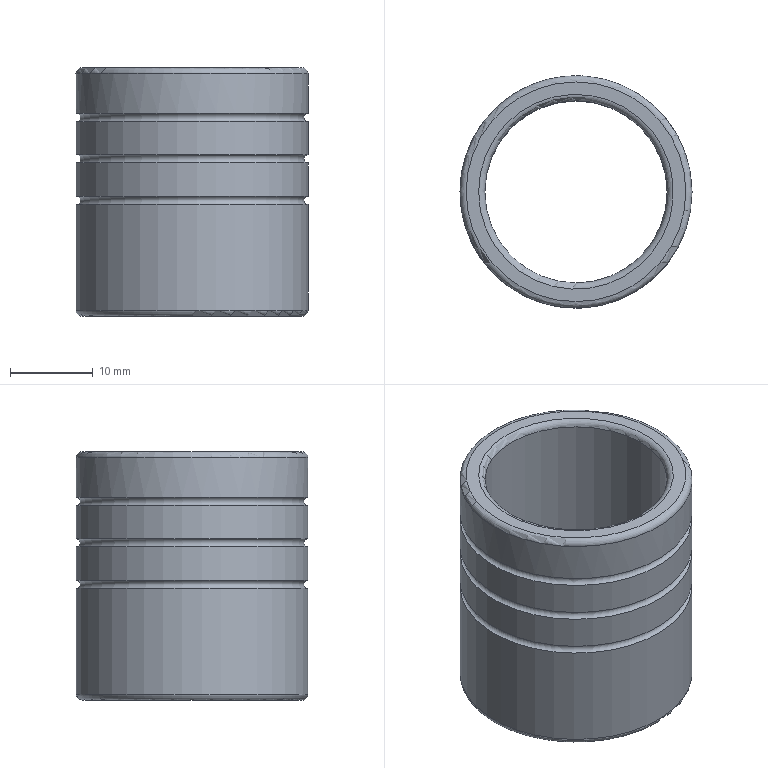Part | STEP file | 200 mesh_id1790 | 1 solid | 14 faces | box 28 x 28 x 30 mm | volume 6929 mm3 | torus 7 | cylinder 5 | plane 2 | commonest cylinder face diameters 28 x4 22 x1
STEP:
#1=CARTESIAN_POINT('',(-17063.884,-4095.269,123.508));
#2=VERTEX_POINT('',#1);
#3=CARTESIAN_POINT('',(-17052.884,-4095.269,123.508));
#4=DIRECTION('',(0.,0.,1.));
#5=DIRECTION('',(-1.,0.,0.));
#6=AXIS2_PLACEMENT_3D('',#3,#4,#5);
#7=CIRCLE('',#6,11.);
#8=EDGE_CURVE('',#2,#2,#7,.T.);
#9=ORIENTED_EDGE('',*,*,#8,.T.);
#10=EDGE_LOOP('',(#9));
#11=FACE_BOUND('',#10,.T.);
#12=CARTESIAN_POINT('',(-17041.884,-4095.269,95.008));
#13=VERTEX_POINT('',#12);
#14=CARTESIAN_POINT('',(-17052.884,-4095.269,95.008));
#15=DIRECTION('',(0.,0.,-1.));
#16=DIRECTION('',(1.,0.,0.));
#17=AXIS2_PLACEMENT_3D('',#14,#15,#16);
#18=CIRCLE('',#17,11.);
#19=EDGE_CURVE('',#13,#13,#18,.T.);
#20=ORIENTED_EDGE('',*,*,#19,.T.);
#21=EDGE_LOOP('',(#20));
#22=FACE_BOUND('',#21,.T.);
#23=CARTESIAN_POINT('',(-17052.884,-4095.269,79.258));
#24=DIRECTION('',(0.,0.,1.));
#25=DIRECTION('',(1.,0.,0.));
#26=AXIS2_PLACEMENT_3D('',#23,#24,#25);
#27=CYLINDRICAL_SURFACE('',#26,11.);
#28=ADVANCED_FACE('',(#11,#22),#27,.F.);
#29=CARTESIAN_POINT('',(-17039.634,-4095.269,94.258));
#30=VERTEX_POINT('',#29);
#31=CARTESIAN_POINT('',(-17052.884,-4095.269,94.258));
#32=DIRECTION('',(0.,0.,-1.));
#33=DIRECTION('',(1.,0.,0.));
#34=AXIS2_PLACEMENT_3D('',#31,#32,#33);
#35=CIRCLE('',#34,13.25);
#36=EDGE_CURVE('',#30,#30,#35,.T.);
#37=ORIENTED_EDGE('',*,*,#36,.T.);
#38=EDGE_LOOP('',(#37));
#39=FACE_BOUND('',#38,.T.);
#40=CARTESIAN_POINT('',(-17041.134,-4095.269,94.258));
#41=VERTEX_POINT('',#40);
#42=CARTESIAN_POINT('',(-17052.884,-4095.269,94.258));
#43=DIRECTION('',(0.,0.,1.));
#44=DIRECTION('',(1.,0.,0.));
#45=AXIS2_PLACEMENT_3D('',#42,#43,#44);
#46=CIRCLE('',#45,11.75);
#47=EDGE_CURVE('',#41,#41,#46,.T.);
#48=ORIENTED_EDGE('',*,*,#47,.T.);
#49=EDGE_LOOP('',(#48));
#50=FACE_BOUND('',#49,.T.);
#51=CARTESIAN_POINT('',(-17063.884,-4095.269,94.258));
#52=DIRECTION('',(0.,0.,1.));
#53=DIRECTION('',(1.,0.,0.));
#54=AXIS2_PLACEMENT_3D('',#51,#52,#53);
#55=PLANE('',#54);
#56=ADVANCED_FACE('',(#39,#50),#55,.F.);
#57=CARTESIAN_POINT('',(-17038.884,-4095.269,95.008));
#58=VERTEX_POINT('',#57);
#59=CARTESIAN_POINT('',(-17052.884,-4095.269,95.008));
#60=DIRECTION('',(0.,0.,1.));
#61=DIRECTION('',(1.,0.,0.));
#62=AXIS2_PLACEMENT_3D('',#59,#60,#61);
#63=CIRCLE('',#62,14.);
#64=EDGE_CURVE('',#58,#58,#63,.T.);
#65=ORIENTED_EDGE('',*,*,#64,.T.);
#66=EDGE_LOOP('',(#65));
#67=FACE_BOUND('',#66,.T.);
#68=CARTESIAN_POINT('',(-17038.884,-4095.269,107.758));
#69=VERTEX_POINT('',#68);
#70=CARTESIAN_POINT('',(-17052.884,-4095.269,107.758));
#71=DIRECTION('',(0.,0.,1.));
#72=DIRECTION('',(1.,0.,0.));
#73=AXIS2_PLACEMENT_3D('',#70,#71,#72);
#74=CIRCLE('',#73,14.);
#75=EDGE_CURVE('',#69,#69,#74,.T.);
#76=ORIENTED_EDGE('',*,*,#75,.F.);
#77=EDGE_LOOP('',(#76));
#78=FACE_BOUND('',#77,.T.);
#79=CARTESIAN_POINT('',(-17052.884,-4095.269,79.258));
#80=DIRECTION('',(0.,0.,1.));
#81=DIRECTION('',(1.,0.,0.));
#82=AXIS2_PLACEMENT_3D('',#79,#80,#81);
#83=CYLINDRICAL_SURFACE('',#82,14.);
#84=ADVANCED_FACE('',(#67,#78),#83,.T.);
#85=CARTESIAN_POINT('',(-17038.884,-4095.269,108.758));
#86=VERTEX_POINT('',#85);
#87=CARTESIAN_POINT('',(-17052.884,-4095.269,108.758));
#88=DIRECTION('',(0.,0.,1.));
#89=DIRECTION('',(1.,0.,0.));
#90=AXIS2_PLACEMENT_3D('',#87,#88,#89);
#91=CIRCLE('',#90,14.);
#92=EDGE_CURVE('',#86,#86,#91,.T.);
#93=ORIENTED_EDGE('',*,*,#92,.F.);
#94=EDGE_LOOP('',(#93));
#95=FACE_BOUND('',#94,.T.);
#96=ORIENTED_EDGE('',*,*,#75,.T.);
#97=EDGE_LOOP('',(#96));
#98=FACE_BOUND('',#97,.T.);
#99=CARTESIAN_POINT('',(-17052.884,-4095.269,108.258));
#100=DIRECTION('',(0.,0.,1.));
#101=DIRECTION('',(1.,0.,0.));
#102=AXIS2_PLACEMENT_3D('',#99,#100,#101);
#103=TOROIDAL_SURFACE('',#102,14.,0.5);
#104=ADVANCED_FACE('',(#95,#98),#103,.F.);
#105=CARTESIAN_POINT('',(-17038.884,-4095.269,112.758));
#106=VERTEX_POINT('',#105);
#107=CARTESIAN_POINT('',(-17052.884,-4095.269,112.758));
#108=DIRECTION('',(0.,0.,1.));
#109=DIRECTION('',(1.,0.,0.));
#110=AXIS2_PLACEMENT_3D('',#107,#108,#109);
#111=CIRCLE('',#110,14.);
#112=EDGE_CURVE('',#106,#106,#111,.T.);
#113=ORIENTED_EDGE('',*,*,#112,.F.);
#114=EDGE_LOOP('',(#113));
#115=FACE_BOUND('',#114,.T.);
#116=ORIENTED_EDGE('',*,*,#92,.T.);
#117=EDGE_LOOP('',(#116));
#118=FACE_BOUND('',#117,.T.);
#119=CARTESIAN_POINT('',(-17052.884,-4095.269,79.258));
#120=DIRECTION('',(0.,0.,1.));
#121=DIRECTION('',(1.,0.,0.));
#122=AXIS2_PLACEMENT_3D('',#119,#120,#121);
#123=CYLINDRICAL_SURFACE('',#122,14.);
#124=ADVANCED_FACE('',(#115,#118),#123,.T.);
#125=CARTESIAN_POINT('',(-17038.884,-4095.269,113.758));
#126=VERTEX_POINT('',#125);
#127=CARTESIAN_POINT('',(-17052.884,-4095.269,113.758));
#128=DIRECTION('',(0.,0.,1.));
#129=DIRECTION('',(1.,0.,0.));
#130=AXIS2_PLACEMENT_3D('',#127,#128,#129);
#131=CIRCLE('',#130,14.);
#132=EDGE_CURVE('',#126,#126,#131,.T.);
#133=ORIENTED_EDGE('',*,*,#132,.F.);
#134=EDGE_LOOP('',(#133));
#135=FACE_BOUND('',#134,.T.);
#136=ORIENTED_EDGE('',*,*,#112,.T.);
#137=EDGE_LOOP('',(#136));
#138=FACE_BOUND('',#137,.T.);
#139=CARTESIAN_POINT('',(-17052.884,-4095.269,113.258));
#140=DIRECTION('',(0.,0.,1.));
#141=DIRECTION('',(1.,0.,0.));
#142=AXIS2_PLACEMENT_3D('',#139,#140,#141);
#143=TOROIDAL_SURFACE('',#142,14.,0.5);
#144=ADVANCED_FACE('',(#135,#138),#143,.F.);
#145=CARTESIAN_POINT('',(-17038.884,-4095.269,117.758));
#146=VERTEX_POINT('',#145);
#147=CARTESIAN_POINT('',(-17052.884,-4095.269,117.758));
#148=DIRECTION('',(0.,0.,1.));
#149=DIRECTION('',(1.,0.,0.));
#150=AXIS2_PLACEMENT_3D('',#147,#148,#149);
#151=CIRCLE('',#150,14.);
#152=EDGE_CURVE('',#146,#146,#151,.T.);
#153=ORIENTED_EDGE('',*,*,#152,.F.);
#154=EDGE_LOOP('',(#153));
#155=FACE_BOUND('',#154,.T.);
#156=ORIENTED_EDGE('',*,*,#132,.T.);
#157=EDGE_LOOP('',(#156));
#158=FACE_BOUND('',#157,.T.);
#159=CARTESIAN_POINT('',(-17052.884,-4095.269,79.258));
#160=DIRECTION('',(0.,0.,1.));
#161=DIRECTION('',(1.,0.,0.));
#162=AXIS2_PLACEMENT_3D('',#159,#160,#161);
#163=CYLINDRICAL_SURFACE('',#162,14.);
#164=ADVANCED_FACE('',(#155,#158),#163,.T.);
#165=CARTESIAN_POINT('',(-17038.884,-4095.269,118.758));
#166=VERTEX_POINT('',#165);
#167=CARTESIAN_POINT('',(-17052.884,-4095.269,118.758));
#168=DIRECTION('',(0.,0.,1.));
#169=DIRECTION('',(1.,0.,0.));
#170=AXIS2_PLACEMENT_3D('',#167,#168,#169);
#171=CIRCLE('',#170,14.);
#172=EDGE_CURVE('',#166,#166,#171,.T.);
#173=ORIENTED_EDGE('',*,*,#172,.F.);
#174=EDGE_LOOP('',(#173));
#175=FACE_BOUND('',#174,.T.);
#176=ORIENTED_EDGE('',*,*,#152,.T.);
#177=EDGE_LOOP('',(#176));
#178=FACE_BOUND('',#177,.T.);
#179=CARTESIAN_POINT('',(-17052.884,-4095.269,118.258));
#180=DIRECTION('',(0.,0.,1.));
#181=DIRECTION('',(1.,0.,0.));
#182=AXIS2_PLACEMENT_3D('',#179,#180,#181);
#183=TOROIDAL_SURFACE('',#182,14.,0.5);
#184=ADVANCED_FACE('',(#175,#178),#183,.F.);
#185=CARTESIAN_POINT('',(-17066.884,-4095.269,123.508));
#186=VERTEX_POINT('',#185);
#187=CARTESIAN_POINT('',(-17052.884,-4095.269,123.508));
#188=DIRECTION('',(0.,0.,-1.));
#189=DIRECTION('',(-1.,0.,0.));
#190=AXIS2_PLACEMENT_3D('',#187,#188,#189);
#191=CIRCLE('',#190,14.);
#192=EDGE_CURVE('',#186,#186,#191,.T.);
#193=ORIENTED_EDGE('',*,*,#192,.T.);
#194=EDGE_LOOP('',(#193));
#195=FACE_BOUND('',#194,.T.);
#196=ORIENTED_EDGE('',*,*,#172,.T.);
#197=EDGE_LOOP('',(#196));
#198=FACE_BOUND('',#197,.T.);
#199=CARTESIAN_POINT('',(-17052.884,-4095.269,79.258));
#200=DIRECTION('',(0.,0.,1.));
#201=DIRECTION('',(1.,0.,0.));
#202=AXIS2_PLACEMENT_3D('',#199,#200,#201);
#203=CYLINDRICAL_SURFACE('',#202,14.);
#204=ADVANCED_FACE('',(#195,#198),#203,.T.);
#205=CARTESIAN_POINT('',(-17064.634,-4095.269,124.258));
#206=VERTEX_POINT('',#205);
#207=CARTESIAN_POINT('',(-17052.884,-4095.269,124.258));
#208=DIRECTION('',(0.,0.,-1.));
#209=DIRECTION('',(-1.,0.,0.));
#210=AXIS2_PLACEMENT_3D('',#207,#208,#209);
#211=CIRCLE('',#210,11.75);
#212=EDGE_CURVE('',#206,#206,#211,.T.);
#213=ORIENTED_EDGE('',*,*,#212,.T.);
#214=EDGE_LOOP('',(#213));
#215=FACE_BOUND('',#214,.T.);
#216=CARTESIAN_POINT('',(-17066.134,-4095.269,124.258));
#217=VERTEX_POINT('',#216);
#218=CARTESIAN_POINT('',(-17052.884,-4095.269,124.258));
#219=DIRECTION('',(0.,0.,1.));
#220=DIRECTION('',(-1.,0.,0.));
#221=AXIS2_PLACEMENT_3D('',#218,#219,#220);
#222=CIRCLE('',#221,13.25);
#223=EDGE_CURVE('',#217,#217,#222,.T.);
#224=ORIENTED_EDGE('',*,*,#223,.T.);
#225=EDGE_LOOP('',(#224));
#226=FACE_BOUND('',#225,.T.);
#227=CARTESIAN_POINT('',(-17066.884,-4095.269,124.258));
#228=DIRECTION('',(0.,0.,-1.));
#229=DIRECTION('',(-1.,0.,0.));
#230=AXIS2_PLACEMENT_3D('',#227,#228,#229);
#231=PLANE('',#230);
#232=ADVANCED_FACE('',(#215,#226),#231,.F.);
#233=ORIENTED_EDGE('',*,*,#36,.F.);
#234=EDGE_LOOP('',(#233));
#235=FACE_BOUND('',#234,.T.);
#236=ORIENTED_EDGE('',*,*,#64,.F.);
#237=EDGE_LOOP('',(#236));
#238=FACE_BOUND('',#237,.T.);
#239=CARTESIAN_POINT('',(-17052.884,-4095.269,95.008));
#240=DIRECTION('',(0.,0.,1.));
#241=DIRECTION('',(1.,0.,0.));
#242=AXIS2_PLACEMENT_3D('',#239,#240,#241);
#243=TOROIDAL_SURFACE('',#242,13.25,0.75);
#244=ADVANCED_FACE('',(#235,#238),#243,.T.);
#245=ORIENTED_EDGE('',*,*,#212,.F.);
#246=EDGE_LOOP('',(#245));
#247=FACE_BOUND('',#246,.T.);
#248=ORIENTED_EDGE('',*,*,#8,.F.);
#249=EDGE_LOOP('',(#248));
#250=FACE_BOUND('',#249,.T.);
#251=CARTESIAN_POINT('',(-17052.884,-4095.269,123.508));
#252=DIRECTION('',(0.,0.,-1.));
#253=DIRECTION('',(-1.,0.,0.));
#254=AXIS2_PLACEMENT_3D('',#251,#252,#253);
#255=TOROIDAL_SURFACE('',#254,11.75,0.75);
#256=ADVANCED_FACE('',(#247,#250),#255,.T.);
#257=ORIENTED_EDGE('',*,*,#192,.F.);
#258=EDGE_LOOP('',(#257));
#259=FACE_BOUND('',#258,.T.);
#260=ORIENTED_EDGE('',*,*,#223,.F.);
#261=EDGE_LOOP('',(#260));
#262=FACE_BOUND('',#261,.T.);
#263=CARTESIAN_POINT('',(-17052.884,-4095.269,123.508));
#264=DIRECTION('',(0.,0.,-1.));
#265=DIRECTION('',(-1.,0.,0.));
#266=AXIS2_PLACEMENT_3D('',#263,#264,#265);
#267=TOROIDAL_SURFACE('',#266,13.25,0.75);
#268=ADVANCED_FACE('',(#259,#262),#267,.T.);
#269=ORIENTED_EDGE('',*,*,#19,.F.);
#270=EDGE_LOOP('',(#269));
#271=FACE_BOUND('',#270,.T.);
#272=ORIENTED_EDGE('',*,*,#47,.F.);
#273=EDGE_LOOP('',(#272));
#274=FACE_BOUND('',#273,.T.);
#275=CARTESIAN_POINT('',(-17052.884,-4095.269,95.008));
#276=DIRECTION('',(0.,0.,1.));
#277=DIRECTION('',(1.,0.,0.));
#278=AXIS2_PLACEMENT_3D('',#275,#276,#277);
#279=TOROIDAL_SURFACE('',#278,11.75,0.75);
#280=ADVANCED_FACE('',(#271,#274),#279,.T.);
#281=CLOSED_SHELL('',(#28,#56,#84,#104,#124,#144,#164,#184,#204,#232,#244,#256,#268,#280));
#282=MANIFOLD_SOLID_BREP('',#281);
#283=(LENGTH_UNIT()NAMED_UNIT(*)SI_UNIT(.MILLI.,.METRE.));
#284=UNCERTAINTY_MEASURE_WITH_UNIT(LENGTH_MEASURE(0.00002),#283,'','');
#285=(NAMED_UNIT(*)PLANE_ANGLE_UNIT()SI_UNIT($,.RADIAN.));
#286=PLANE_ANGLE_MEASURE_WITH_UNIT(PLANE_ANGLE_MEASURE(0.01745),#285);
#287=DIMENSIONAL_EXPONENTS(0.,0.,0.,0.,0.,0.,0.);
#288=(CONVERSION_BASED_UNIT('DEGREE',#286)NAMED_UNIT(#287)PLANE_ANGLE_UNIT());
#289=(NAMED_UNIT(*)SI_UNIT($,.STERADIAN.)SOLID_ANGLE_UNIT());
#290=(GEOMETRIC_REPRESENTATION_CONTEXT(3)GLOBAL_UNCERTAINTY_ASSIGNED_CONTEXT((#284))GLOBAL_UNIT_ASSIGNED_CONTEXT((#283,#288,#289))REPRESENTATION_CONTEXT('',''));
#291=ADVANCED_BREP_SHAPE_REPRESENTATION('',(#282),#290);